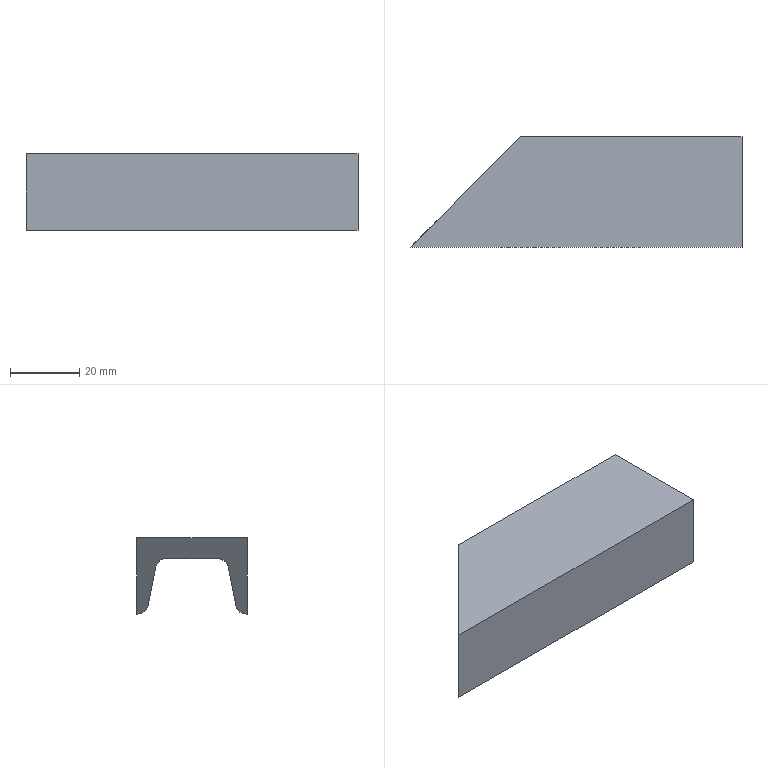Part | NX | features solid 2 | 1 solid | 14 faces | box 96 x 32 x 22 mm | volume 26641 mm3 | plane 10 | cylinder 4 | commonest cylinder face diameters 6 x4
STEP:
#1=CARTESIAN_POINT('',(-60.648,319.567,62.866));
#2=VERTEX_POINT('',#1);
#3=CARTESIAN_POINT('',(-61.,319.216,62.866));
#4=VERTEX_POINT('',#3);
#5=CARTESIAN_POINT('',(-22.5,357.716,62.866));
#6=DIRECTION('',(-0.7071,-0.7071,0.));
#7=VECTOR('',#6,1000.);
#8=LINE('',#5,#7);
#9=EDGE_CURVE('',#2,#4,#8,.T.);
#10=ORIENTED_EDGE('',*,*,#9,.F.);
#11=CARTESIAN_POINT('',(35.,319.567,62.866));
#12=VERTEX_POINT('',#11);
#13=CARTESIAN_POINT('',(-13.,319.567,62.866));
#14=DIRECTION('',(-1.,0.,0.));
#15=VECTOR('',#14,1000.);
#16=LINE('',#13,#15);
#17=EDGE_CURVE('',#2,#12,#16,.F.);
#18=ORIENTED_EDGE('',*,*,#17,.T.);
#19=CARTESIAN_POINT('',(35.,319.216,62.866));
#20=VERTEX_POINT('',#19);
#21=CARTESIAN_POINT('',(35.,335.216,62.866));
#22=DIRECTION('',(0.,1.,0.));
#23=VECTOR('',#22,1000.);
#24=LINE('',#21,#23);
#25=EDGE_CURVE('',#20,#12,#24,.T.);
#26=ORIENTED_EDGE('',*,*,#25,.F.);
#27=CARTESIAN_POINT('',(-0.000000942,319.216,62.866));
#28=DIRECTION('',(1.,0.,0.));
#29=VECTOR('',#28,1000.);
#30=LINE('',#27,#29);
#31=EDGE_CURVE('',#4,#20,#30,.T.);
#32=ORIENTED_EDGE('',*,*,#31,.F.);
#33=EDGE_LOOP('',(#10,#18,#26,#32));
#34=FACE_BOUND('',#33,.T.);
#35=CARTESIAN_POINT('',(-0.000000942,335.216,62.866));
#36=DIRECTION('',(0.,0.,-1.));
#37=DIRECTION('',(-1.,0.,0.));
#38=AXIS2_PLACEMENT_3D('',#35,#36,#37);
#39=PLANE('',#38);
#40=ADVANCED_FACE('',(#34),#39,.T.);
#41=CARTESIAN_POINT('',(-29.,351.216,62.866));
#42=VERTEX_POINT('',#41);
#43=CARTESIAN_POINT('',(-29.352,350.864,62.866));
#44=VERTEX_POINT('',#43);
#45=CARTESIAN_POINT('',(-22.5,357.716,62.866));
#46=DIRECTION('',(-0.7071,-0.7071,0.));
#47=VECTOR('',#46,1000.);
#48=LINE('',#45,#47);
#49=EDGE_CURVE('',#42,#44,#48,.T.);
#50=ORIENTED_EDGE('',*,*,#49,.F.);
#51=CARTESIAN_POINT('',(35.,351.216,62.866));
#52=VERTEX_POINT('',#51);
#53=CARTESIAN_POINT('',(-0.000000942,351.216,62.866));
#54=DIRECTION('',(-1.,0.,0.));
#55=VECTOR('',#54,1000.);
#56=LINE('',#53,#55);
#57=EDGE_CURVE('',#52,#42,#56,.T.);
#58=ORIENTED_EDGE('',*,*,#57,.F.);
#59=CARTESIAN_POINT('',(35.,350.864,62.866));
#60=VERTEX_POINT('',#59);
#61=CARTESIAN_POINT('',(35.,335.216,62.866));
#62=DIRECTION('',(0.,1.,0.));
#63=VECTOR('',#62,1000.);
#64=LINE('',#61,#63);
#65=EDGE_CURVE('',#60,#52,#64,.T.);
#66=ORIENTED_EDGE('',*,*,#65,.F.);
#67=CARTESIAN_POINT('',(-0.000000942,350.864,62.866));
#68=DIRECTION('',(-1.,0.,0.));
#69=VECTOR('',#68,1000.);
#70=LINE('',#67,#69);
#71=EDGE_CURVE('',#60,#44,#70,.T.);
#72=ORIENTED_EDGE('',*,*,#71,.T.);
#73=EDGE_LOOP('',(#50,#58,#66,#72));
#74=FACE_BOUND('',#73,.T.);
#75=CARTESIAN_POINT('',(-0.000000942,335.216,62.866));
#76=DIRECTION('',(0.,0.,-1.));
#77=DIRECTION('',(-1.,0.,0.));
#78=AXIS2_PLACEMENT_3D('',#75,#76,#77);
#79=PLANE('',#78);
#80=ADVANCED_FACE('',(#74),#79,.T.);
#81=CARTESIAN_POINT('',(-61.,319.216,84.866));
#82=VERTEX_POINT('',#81);
#83=CARTESIAN_POINT('',(-29.,351.216,84.866));
#84=VERTEX_POINT('',#83);
#85=CARTESIAN_POINT('',(-22.5,357.716,84.866));
#86=DIRECTION('',(0.7071,0.7071,0.));
#87=VECTOR('',#86,1000.);
#88=LINE('',#85,#87);
#89=EDGE_CURVE('',#82,#84,#88,.T.);
#90=ORIENTED_EDGE('',*,*,#89,.F.);
#91=CARTESIAN_POINT('',(35.,319.216,84.866));
#92=VERTEX_POINT('',#91);
#93=CARTESIAN_POINT('',(-0.000000942,319.216,84.866));
#94=DIRECTION('',(-1.,0.,0.));
#95=VECTOR('',#94,1000.);
#96=LINE('',#93,#95);
#97=EDGE_CURVE('',#92,#82,#96,.T.);
#98=ORIENTED_EDGE('',*,*,#97,.F.);
#99=CARTESIAN_POINT('',(35.,351.216,84.866));
#100=VERTEX_POINT('',#99);
#101=CARTESIAN_POINT('',(35.,335.216,84.866));
#102=DIRECTION('',(0.,-1.,0.));
#103=VECTOR('',#102,1000.);
#104=LINE('',#101,#103);
#105=EDGE_CURVE('',#100,#92,#104,.T.);
#106=ORIENTED_EDGE('',*,*,#105,.F.);
#107=CARTESIAN_POINT('',(-0.000000942,351.216,84.866));
#108=DIRECTION('',(1.,0.,0.));
#109=VECTOR('',#108,1000.);
#110=LINE('',#107,#109);
#111=EDGE_CURVE('',#84,#100,#110,.T.);
#112=ORIENTED_EDGE('',*,*,#111,.F.);
#113=EDGE_LOOP('',(#90,#98,#106,#112));
#114=FACE_BOUND('',#113,.T.);
#115=CARTESIAN_POINT('',(-0.000000942,335.216,84.866));
#116=DIRECTION('',(0.,0.,1.));
#117=DIRECTION('',(1.,0.,0.));
#118=AXIS2_PLACEMENT_3D('',#115,#116,#117);
#119=PLANE('',#118);
#120=ADVANCED_FACE('',(#114),#119,.T.);
#121=CARTESIAN_POINT('',(35.,319.216,74.866));
#122=DIRECTION('',(0.,0.,1.));
#123=VECTOR('',#122,1000.);
#124=LINE('',#121,#123);
#125=EDGE_CURVE('',#20,#92,#124,.T.);
#126=ORIENTED_EDGE('',*,*,#125,.T.);
#127=ORIENTED_EDGE('',*,*,#97,.T.);
#128=CARTESIAN_POINT('',(-61.,319.216,84.));
#129=DIRECTION('',(0.,0.,-1.));
#130=VECTOR('',#129,1000.);
#131=LINE('',#128,#130);
#132=EDGE_CURVE('',#4,#82,#131,.F.);
#133=ORIENTED_EDGE('',*,*,#132,.F.);
#134=ORIENTED_EDGE('',*,*,#31,.T.);
#135=EDGE_LOOP('',(#126,#127,#133,#134));
#136=FACE_BOUND('',#135,.T.);
#137=CARTESIAN_POINT('',(-0.000000942,319.216,74.866));
#138=DIRECTION('',(0.,-1.,0.));
#139=DIRECTION('',(0.,0.,-1.));
#140=AXIS2_PLACEMENT_3D('',#137,#138,#139);
#141=PLANE('',#140);
#142=ADVANCED_FACE('',(#136),#141,.T.);
#143=CARTESIAN_POINT('',(-29.,351.216,74.866));
#144=DIRECTION('',(0.,0.,-1.));
#145=VECTOR('',#144,1000.);
#146=LINE('',#143,#145);
#147=EDGE_CURVE('',#84,#42,#146,.T.);
#148=ORIENTED_EDGE('',*,*,#147,.F.);
#149=ORIENTED_EDGE('',*,*,#111,.T.);
#150=CARTESIAN_POINT('',(35.,351.216,74.866));
#151=DIRECTION('',(0.,0.,1.));
#152=VECTOR('',#151,1000.);
#153=LINE('',#150,#152);
#154=EDGE_CURVE('',#52,#100,#153,.T.);
#155=ORIENTED_EDGE('',*,*,#154,.F.);
#156=ORIENTED_EDGE('',*,*,#57,.T.);
#157=EDGE_LOOP('',(#148,#149,#155,#156));
#158=FACE_BOUND('',#157,.T.);
#159=CARTESIAN_POINT('',(-0.000000942,351.216,74.866));
#160=DIRECTION('',(0.,1.,0.));
#161=DIRECTION('',(0.,0.,1.));
#162=AXIS2_PLACEMENT_3D('',#159,#160,#161);
#163=PLANE('',#162);
#164=ADVANCED_FACE('',(#158),#163,.T.);
#165=ORIENTED_EDGE('',*,*,#25,.T.);
#166=CARTESIAN_POINT('',(35.,322.51,65.28));
#167=VERTEX_POINT('',#166);
#168=CARTESIAN_POINT('',(35.,319.567,65.866));
#169=DIRECTION('',(1.,0.,0.));
#170=DIRECTION('',(0.,0.,-1.));
#171=AXIS2_PLACEMENT_3D('',#168,#169,#170);
#172=CIRCLE('',#171,3.);
#173=EDGE_CURVE('',#12,#167,#172,.T.);
#174=ORIENTED_EDGE('',*,*,#173,.T.);
#175=CARTESIAN_POINT('',(35.,324.735,76.452));
#176=VERTEX_POINT('',#175);
#177=CARTESIAN_POINT('',(35.,322.859,67.036));
#178=DIRECTION('',(0.,0.1953,0.9807));
#179=VECTOR('',#178,1000.);
#180=LINE('',#177,#179);
#181=EDGE_CURVE('',#167,#176,#180,.T.);
#182=ORIENTED_EDGE('',*,*,#181,.T.);
#183=CARTESIAN_POINT('',(35.,327.677,78.866));
#184=VERTEX_POINT('',#183);
#185=CARTESIAN_POINT('',(35.,327.677,75.866));
#186=DIRECTION('',(1.,0.,0.));
#187=DIRECTION('',(0.,0.,-1.));
#188=AXIS2_PLACEMENT_3D('',#185,#186,#187);
#189=CIRCLE('',#188,3.);
#190=EDGE_CURVE('',#176,#184,#189,.F.);
#191=ORIENTED_EDGE('',*,*,#190,.T.);
#192=CARTESIAN_POINT('',(35.,342.754,78.866));
#193=VERTEX_POINT('',#192);
#194=CARTESIAN_POINT('',(35.,335.216,78.866));
#195=DIRECTION('',(0.,-1.,0.));
#196=VECTOR('',#195,1000.);
#197=LINE('',#194,#196);
#198=EDGE_CURVE('',#193,#184,#197,.T.);
#199=ORIENTED_EDGE('',*,*,#198,.F.);
#200=CARTESIAN_POINT('',(35.,345.697,76.452));
#201=VERTEX_POINT('',#200);
#202=CARTESIAN_POINT('',(35.,342.754,75.866));
#203=DIRECTION('',(1.,0.,0.));
#204=DIRECTION('',(0.,0.,-1.));
#205=AXIS2_PLACEMENT_3D('',#202,#203,#204);
#206=CIRCLE('',#205,3.);
#207=EDGE_CURVE('',#193,#201,#206,.F.);
#208=ORIENTED_EDGE('',*,*,#207,.T.);
#209=CARTESIAN_POINT('',(35.,347.922,65.28));
#210=VERTEX_POINT('',#209);
#211=CARTESIAN_POINT('',(35.,345.743,76.221));
#212=DIRECTION('',(0.,-0.1953,0.9807));
#213=VECTOR('',#212,1000.);
#214=LINE('',#211,#213);
#215=EDGE_CURVE('',#210,#201,#214,.T.);
#216=ORIENTED_EDGE('',*,*,#215,.F.);
#217=CARTESIAN_POINT('',(35.,350.864,65.866));
#218=DIRECTION('',(1.,0.,0.));
#219=DIRECTION('',(0.,0.,-1.));
#220=AXIS2_PLACEMENT_3D('',#217,#218,#219);
#221=CIRCLE('',#220,3.);
#222=EDGE_CURVE('',#210,#60,#221,.T.);
#223=ORIENTED_EDGE('',*,*,#222,.T.);
#224=ORIENTED_EDGE('',*,*,#65,.T.);
#225=ORIENTED_EDGE('',*,*,#154,.T.);
#226=ORIENTED_EDGE('',*,*,#105,.T.);
#227=ORIENTED_EDGE('',*,*,#125,.F.);
#228=EDGE_LOOP('',(#165,#174,#182,#191,#199,#208,#216,#223,#224,#225,#226,#227));
#229=FACE_BOUND('',#228,.T.);
#230=CARTESIAN_POINT('',(35.,335.216,74.866));
#231=DIRECTION('',(1.,0.,0.));
#232=DIRECTION('',(0.,0.,-1.));
#233=AXIS2_PLACEMENT_3D('',#230,#231,#232);
#234=PLANE('',#233);
#235=ADVANCED_FACE('',(#229),#234,.T.);
#236=CARTESIAN_POINT('',(-52.539,327.677,78.866));
#237=VERTEX_POINT('',#236);
#238=CARTESIAN_POINT('',(-61.,327.677,78.866));
#239=DIRECTION('',(-1.,0.,0.));
#240=VECTOR('',#239,1000.);
#241=LINE('',#238,#240);
#242=EDGE_CURVE('',#184,#237,#241,.T.);
#243=ORIENTED_EDGE('',*,*,#242,.T.);
#244=CARTESIAN_POINT('',(-37.461,342.754,78.866));
#245=VERTEX_POINT('',#244);
#246=CARTESIAN_POINT('',(-22.5,357.716,78.866));
#247=DIRECTION('',(0.7071,0.7071,0.));
#248=VECTOR('',#247,1000.);
#249=LINE('',#246,#248);
#250=EDGE_CURVE('',#237,#245,#249,.T.);
#251=ORIENTED_EDGE('',*,*,#250,.T.);
#252=CARTESIAN_POINT('',(35.,342.754,78.866));
#253=DIRECTION('',(1.,0.,0.));
#254=VECTOR('',#253,1000.);
#255=LINE('',#252,#254);
#256=EDGE_CURVE('',#245,#193,#255,.T.);
#257=ORIENTED_EDGE('',*,*,#256,.T.);
#258=ORIENTED_EDGE('',*,*,#198,.T.);
#259=EDGE_LOOP('',(#243,#251,#257,#258));
#260=FACE_BOUND('',#259,.T.);
#261=CARTESIAN_POINT('',(-0.000000942,335.216,78.866));
#262=DIRECTION('',(0.,0.,1.));
#263=DIRECTION('',(1.,0.,0.));
#264=AXIS2_PLACEMENT_3D('',#261,#262,#263);
#265=PLANE('',#264);
#266=ADVANCED_FACE('',(#260),#265,.F.);
#267=CARTESIAN_POINT('',(-57.706,322.51,65.28));
#268=VERTEX_POINT('',#267);
#269=CARTESIAN_POINT('',(-13.,322.51,65.28));
#270=DIRECTION('',(-1.,0.,0.));
#271=VECTOR('',#270,1000.);
#272=LINE('',#269,#271);
#273=EDGE_CURVE('',#167,#268,#272,.T.);
#274=ORIENTED_EDGE('',*,*,#273,.T.);
#275=CARTESIAN_POINT('',(-55.481,324.735,76.452));
#276=VERTEX_POINT('',#275);
#277=CARTESIAN_POINT('',(-55.726,324.49,75.222));
#278=DIRECTION('',(0.1917,0.1917,0.9625));
#279=VECTOR('',#278,1000.);
#280=LINE('',#277,#279);
#281=EDGE_CURVE('',#268,#276,#280,.T.);
#282=ORIENTED_EDGE('',*,*,#281,.T.);
#283=CARTESIAN_POINT('',(-0.000000942,324.735,76.452));
#284=DIRECTION('',(-1.,0.,0.));
#285=VECTOR('',#284,1000.);
#286=LINE('',#283,#285);
#287=EDGE_CURVE('',#276,#176,#286,.F.);
#288=ORIENTED_EDGE('',*,*,#287,.T.);
#289=ORIENTED_EDGE('',*,*,#181,.F.);
#290=EDGE_LOOP('',(#274,#282,#288,#289));
#291=FACE_BOUND('',#290,.T.);
#292=CARTESIAN_POINT('',(-13.,322.859,67.036));
#293=DIRECTION('',(0.,-0.9807,0.1953));
#294=DIRECTION('',(0.,-0.1953,-0.9807));
#295=AXIS2_PLACEMENT_3D('',#292,#293,#294);
#296=PLANE('',#295);
#297=ADVANCED_FACE('',(#291),#296,.F.);
#298=CARTESIAN_POINT('',(-34.519,345.697,76.452));
#299=VERTEX_POINT('',#298);
#300=CARTESIAN_POINT('',(-0.000000942,345.697,76.452));
#301=DIRECTION('',(1.,0.,0.));
#302=VECTOR('',#301,1000.);
#303=LINE('',#300,#302);
#304=EDGE_CURVE('',#201,#299,#303,.F.);
#305=ORIENTED_EDGE('',*,*,#304,.T.);
#306=CARTESIAN_POINT('',(-32.294,347.922,65.28));
#307=VERTEX_POINT('',#306);
#308=CARTESIAN_POINT('',(-31.922,348.294,63.411));
#309=DIRECTION('',(0.1917,0.1917,-0.9625));
#310=VECTOR('',#309,1000.);
#311=LINE('',#308,#310);
#312=EDGE_CURVE('',#299,#307,#311,.T.);
#313=ORIENTED_EDGE('',*,*,#312,.T.);
#314=CARTESIAN_POINT('',(-0.000000942,347.922,65.28));
#315=DIRECTION('',(-1.,0.,0.));
#316=VECTOR('',#315,1000.);
#317=LINE('',#314,#316);
#318=EDGE_CURVE('',#307,#210,#317,.F.);
#319=ORIENTED_EDGE('',*,*,#318,.T.);
#320=ORIENTED_EDGE('',*,*,#215,.T.);
#321=EDGE_LOOP('',(#305,#313,#319,#320));
#322=FACE_BOUND('',#321,.T.);
#323=CARTESIAN_POINT('',(-13.,347.572,67.036));
#324=DIRECTION('',(0.,0.9807,0.1953));
#325=DIRECTION('',(0.,-0.1953,0.9807));
#326=AXIS2_PLACEMENT_3D('',#323,#324,#325);
#327=PLANE('',#326);
#328=ADVANCED_FACE('',(#322),#327,.F.);
#329=CARTESIAN_POINT('',(-60.648,319.567,65.866));
#330=DIRECTION('',(0.7071,-0.7071,0.));
#331=DIRECTION('',(0.7071,0.7071,0.));
#332=AXIS2_PLACEMENT_3D('',#329,#330,#331);
#333=ELLIPSE('',#332,4.243,3.);
#334=EDGE_CURVE('',#268,#2,#333,.F.);
#335=ORIENTED_EDGE('',*,*,#334,.F.);
#336=ORIENTED_EDGE('',*,*,#273,.F.);
#337=ORIENTED_EDGE('',*,*,#173,.F.);
#338=ORIENTED_EDGE('',*,*,#17,.F.);
#339=EDGE_LOOP('',(#335,#336,#337,#338));
#340=FACE_BOUND('',#339,.T.);
#341=CARTESIAN_POINT('',(-13.,319.567,65.866));
#342=DIRECTION('',(1.,0.,0.));
#343=DIRECTION('',(0.,1.,0.));
#344=AXIS2_PLACEMENT_3D('',#341,#342,#343);
#345=CYLINDRICAL_SURFACE('',#344,3.);
#346=ADVANCED_FACE('',(#340),#345,.T.);
#347=CARTESIAN_POINT('',(-29.352,350.864,65.866));
#348=DIRECTION('',(0.7071,-0.7071,0.));
#349=DIRECTION('',(0.7071,0.7071,0.));
#350=AXIS2_PLACEMENT_3D('',#347,#348,#349);
#351=ELLIPSE('',#350,4.243,3.);
#352=EDGE_CURVE('',#44,#307,#351,.F.);
#353=ORIENTED_EDGE('',*,*,#352,.F.);
#354=ORIENTED_EDGE('',*,*,#71,.F.);
#355=ORIENTED_EDGE('',*,*,#222,.F.);
#356=ORIENTED_EDGE('',*,*,#318,.F.);
#357=EDGE_LOOP('',(#353,#354,#355,#356));
#358=FACE_BOUND('',#357,.T.);
#359=CARTESIAN_POINT('',(-0.000000942,350.864,65.866));
#360=DIRECTION('',(1.,0.,0.));
#361=DIRECTION('',(0.,1.,0.));
#362=AXIS2_PLACEMENT_3D('',#359,#360,#361);
#363=CYLINDRICAL_SURFACE('',#362,3.);
#364=ADVANCED_FACE('',(#358),#363,.T.);
#365=ORIENTED_EDGE('',*,*,#256,.F.);
#366=CARTESIAN_POINT('',(-37.461,342.754,75.866));
#367=DIRECTION('',(0.7071,-0.7071,0.));
#368=DIRECTION('',(-0.7071,-0.7071,0.));
#369=AXIS2_PLACEMENT_3D('',#366,#367,#368);
#370=ELLIPSE('',#369,4.243,3.);
#371=EDGE_CURVE('',#245,#299,#370,.F.);
#372=ORIENTED_EDGE('',*,*,#371,.T.);
#373=ORIENTED_EDGE('',*,*,#304,.F.);
#374=ORIENTED_EDGE('',*,*,#207,.F.);
#375=EDGE_LOOP('',(#365,#372,#373,#374));
#376=FACE_BOUND('',#375,.T.);
#377=CARTESIAN_POINT('',(-0.000000942,342.754,75.866));
#378=DIRECTION('',(-1.,0.,0.));
#379=DIRECTION('',(0.,-1.,0.));
#380=AXIS2_PLACEMENT_3D('',#377,#378,#379);
#381=CYLINDRICAL_SURFACE('',#380,3.);
#382=ADVANCED_FACE('',(#376),#381,.F.);
#383=ORIENTED_EDGE('',*,*,#287,.F.);
#384=CARTESIAN_POINT('',(-52.539,327.677,75.866));
#385=DIRECTION('',(0.7071,-0.7071,0.));
#386=DIRECTION('',(0.7071,0.7071,0.));
#387=AXIS2_PLACEMENT_3D('',#384,#385,#386);
#388=ELLIPSE('',#387,4.243,3.);
#389=EDGE_CURVE('',#276,#237,#388,.F.);
#390=ORIENTED_EDGE('',*,*,#389,.T.);
#391=ORIENTED_EDGE('',*,*,#242,.F.);
#392=ORIENTED_EDGE('',*,*,#190,.F.);
#393=EDGE_LOOP('',(#383,#390,#391,#392));
#394=FACE_BOUND('',#393,.T.);
#395=CARTESIAN_POINT('',(-0.000000942,327.677,75.866));
#396=DIRECTION('',(1.,0.,0.));
#397=DIRECTION('',(0.,1.,0.));
#398=AXIS2_PLACEMENT_3D('',#395,#396,#397);
#399=CYLINDRICAL_SURFACE('',#398,3.);
#400=ADVANCED_FACE('',(#394),#399,.F.);
#401=ORIENTED_EDGE('',*,*,#89,.T.);
#402=ORIENTED_EDGE('',*,*,#147,.T.);
#403=ORIENTED_EDGE('',*,*,#49,.T.);
#404=ORIENTED_EDGE('',*,*,#352,.T.);
#405=ORIENTED_EDGE('',*,*,#312,.F.);
#406=ORIENTED_EDGE('',*,*,#371,.F.);
#407=ORIENTED_EDGE('',*,*,#250,.F.);
#408=ORIENTED_EDGE('',*,*,#389,.F.);
#409=ORIENTED_EDGE('',*,*,#281,.F.);
#410=ORIENTED_EDGE('',*,*,#334,.T.);
#411=ORIENTED_EDGE('',*,*,#9,.T.);
#412=ORIENTED_EDGE('',*,*,#132,.T.);
#413=EDGE_LOOP('',(#401,#402,#403,#404,#405,#406,#407,#408,#409,#410,#411,#412));
#414=FACE_BOUND('',#413,.T.);
#415=CARTESIAN_POINT('',(-29.,351.216,0.5));
#416=DIRECTION('',(0.7071,-0.7071,0.));
#417=DIRECTION('',(0.7071,0.7071,0.));
#418=AXIS2_PLACEMENT_3D('',#415,#416,#417);
#419=PLANE('',#418);
#420=ADVANCED_FACE('',(#414),#419,.F.);
#421=CLOSED_SHELL('',(#40,#80,#120,#142,#164,#235,#266,#297,#328,#346,#364,#382,#400,#420));
#422=MANIFOLD_SOLID_BREP('',#421);
#423=(LENGTH_UNIT()NAMED_UNIT(*)SI_UNIT(.MILLI.,.METRE.));
#424=UNCERTAINTY_MEASURE_WITH_UNIT(LENGTH_MEASURE(0.00001),#423,'','');
#425=(NAMED_UNIT(*)PLANE_ANGLE_UNIT()SI_UNIT($,.RADIAN.));
#426=(NAMED_UNIT(*)SI_UNIT($,.STERADIAN.)SOLID_ANGLE_UNIT());
#427=(GEOMETRIC_REPRESENTATION_CONTEXT(3)GLOBAL_UNCERTAINTY_ASSIGNED_CONTEXT((#424))GLOBAL_UNIT_ASSIGNED_CONTEXT((#423,#425,#426))REPRESENTATION_CONTEXT('',''));
#428=ADVANCED_BREP_SHAPE_REPRESENTATION('',(#422),#427);